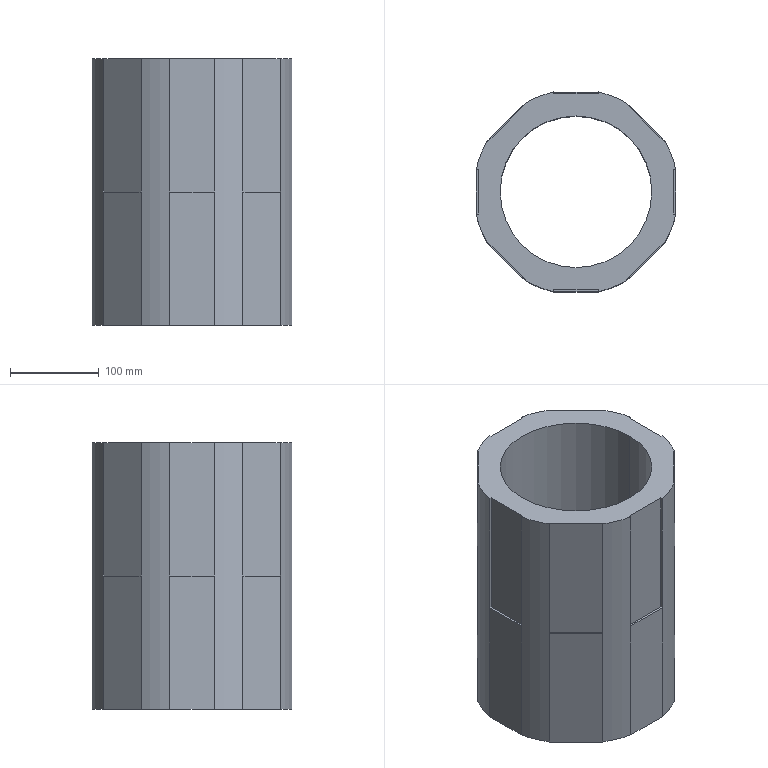Part | SolidWorks | features BaseBody 1 | 1 solid | 52 faces | box 224.499 x 224.499 x 300 mm | volume 5216561 mm3 | plane 42 | cylinder 10 | commonest cylinder face diameters 230 x8 170.4 x2
STEP:
#1=CARTESIAN_POINT('',(2951.757,1619.154,150.));
#2=VERTEX_POINT('',#1);
#3=CARTESIAN_POINT('',(3122.157,1619.154,150.));
#4=VERTEX_POINT('',#3);
#5=CARTESIAN_POINT('',(3036.957,1619.154,150.));
#6=DIRECTION('',(0.,0.,1.));
#7=DIRECTION('',(1.,0.,0.));
#8=AXIS2_PLACEMENT_3D('',#5,#6,#7);
#9=CIRCLE('',#8,85.2);
#10=EDGE_CURVE('',#2,#4,#9,.T.);
#11=ORIENTED_EDGE('',*,*,#10,.T.);
#12=CARTESIAN_POINT('',(3122.157,1619.154,-150.));
#13=VERTEX_POINT('',#12);
#14=CARTESIAN_POINT('',(3122.157,1619.154,150.));
#15=DIRECTION('',(0.,0.,-1.));
#16=VECTOR('',#15,1000.);
#17=LINE('',#14,#16);
#18=EDGE_CURVE('',#4,#13,#17,.T.);
#19=ORIENTED_EDGE('',*,*,#18,.T.);
#20=CARTESIAN_POINT('',(2951.757,1619.154,-150.));
#21=VERTEX_POINT('',#20);
#22=CARTESIAN_POINT('',(3036.957,1619.154,-150.));
#23=DIRECTION('',(0.,0.,1.));
#24=DIRECTION('',(1.,0.,0.));
#25=AXIS2_PLACEMENT_3D('',#22,#23,#24);
#26=CIRCLE('',#25,85.2);
#27=EDGE_CURVE('',#21,#13,#26,.T.);
#28=ORIENTED_EDGE('',*,*,#27,.F.);
#29=CARTESIAN_POINT('',(2951.757,1619.154,150.));
#30=DIRECTION('',(0.,0.,-1.));
#31=VECTOR('',#30,1000.);
#32=LINE('',#29,#31);
#33=EDGE_CURVE('',#2,#21,#32,.T.);
#34=ORIENTED_EDGE('',*,*,#33,.F.);
#35=EDGE_LOOP('',(#11,#19,#28,#34));
#36=FACE_OUTER_BOUND('',#35,.T.);
#37=CARTESIAN_POINT('',(3036.957,1619.154,150.));
#38=DIRECTION('',(0.,0.,-1.));
#39=DIRECTION('',(-1.,0.,0.));
#40=AXIS2_PLACEMENT_3D('',#37,#38,#39);
#41=CYLINDRICAL_SURFACE('',#40,85.2);
#42=ADVANCED_FACE('',(#36),#41,.F.);
#43=CARTESIAN_POINT('',(2979.668,1718.869,0.));
#44=VERTEX_POINT('',#43);
#45=CARTESIAN_POINT('',(2980.388,1718.149,0.));
#46=VERTEX_POINT('',#45);
#47=CARTESIAN_POINT('',(2979.668,1718.869,0.));
#48=DIRECTION('',(0.7071,-0.7071,0.));
#49=VECTOR('',#48,1000.);
#50=LINE('',#47,#49);
#51=EDGE_CURVE('',#44,#46,#50,.T.);
#52=ORIENTED_EDGE('',*,*,#51,.T.);
#53=CARTESIAN_POINT('',(2980.388,1718.149,150.));
#54=VERTEX_POINT('',#53);
#55=CARTESIAN_POINT('',(2980.388,1718.149,150.));
#56=DIRECTION('',(0.,0.,-1.));
#57=VECTOR('',#56,1000.);
#58=LINE('',#55,#57);
#59=EDGE_CURVE('',#54,#46,#58,.T.);
#60=ORIENTED_EDGE('',*,*,#59,.F.);
#61=CARTESIAN_POINT('',(2979.668,1718.869,150.));
#62=VERTEX_POINT('',#61);
#63=CARTESIAN_POINT('',(2979.668,1718.869,150.));
#64=DIRECTION('',(0.7071,-0.7071,0.));
#65=VECTOR('',#64,1000.);
#66=LINE('',#63,#65);
#67=EDGE_CURVE('',#62,#54,#66,.T.);
#68=ORIENTED_EDGE('',*,*,#67,.F.);
#69=CARTESIAN_POINT('',(2979.668,1718.869,150.));
#70=DIRECTION('',(0.,0.,-1.));
#71=VECTOR('',#70,1000.);
#72=LINE('',#69,#71);
#73=EDGE_CURVE('',#62,#44,#72,.T.);
#74=ORIENTED_EDGE('',*,*,#73,.T.);
#75=EDGE_LOOP('',(#52,#60,#68,#74));
#76=FACE_OUTER_BOUND('',#75,.T.);
#77=CARTESIAN_POINT('',(2979.668,1718.869,150.));
#78=DIRECTION('',(0.7071,0.7071,0.));
#79=DIRECTION('',(-0.7071,0.7071,0.));
#80=AXIS2_PLACEMENT_3D('',#77,#78,#79);
#81=PLANE('',#80);
#82=ADVANCED_FACE('',(#76),#81,.F.);
#83=CARTESIAN_POINT('',(2937.962,1675.723,0.));
#84=VERTEX_POINT('',#83);
#85=CARTESIAN_POINT('',(2980.388,1718.149,0.));
#86=DIRECTION('',(-0.7071,-0.7071,0.));
#87=VECTOR('',#86,1000.);
#88=LINE('',#85,#87);
#89=EDGE_CURVE('',#46,#84,#88,.T.);
#90=ORIENTED_EDGE('',*,*,#89,.T.);
#91=CARTESIAN_POINT('',(2937.962,1675.723,150.));
#92=VERTEX_POINT('',#91);
#93=CARTESIAN_POINT('',(2937.962,1675.723,150.));
#94=DIRECTION('',(0.,0.,-1.));
#95=VECTOR('',#94,1000.);
#96=LINE('',#93,#95);
#97=EDGE_CURVE('',#92,#84,#96,.T.);
#98=ORIENTED_EDGE('',*,*,#97,.F.);
#99=CARTESIAN_POINT('',(2980.388,1718.149,150.));
#100=DIRECTION('',(-0.7071,-0.7071,0.));
#101=VECTOR('',#100,1000.);
#102=LINE('',#99,#101);
#103=EDGE_CURVE('',#54,#92,#102,.T.);
#104=ORIENTED_EDGE('',*,*,#103,.F.);
#105=ORIENTED_EDGE('',*,*,#59,.T.);
#106=EDGE_LOOP('',(#90,#98,#104,#105));
#107=FACE_OUTER_BOUND('',#106,.T.);
#108=CARTESIAN_POINT('',(2980.388,1718.149,150.));
#109=DIRECTION('',(0.7071,-0.7071,0.));
#110=DIRECTION('',(0.7071,0.7071,0.));
#111=AXIS2_PLACEMENT_3D('',#108,#109,#110);
#112=PLANE('',#111);
#113=ADVANCED_FACE('',(#107),#112,.F.);
#114=CARTESIAN_POINT('',(2937.242,1676.443,0.));
#115=VERTEX_POINT('',#114);
#116=CARTESIAN_POINT('',(2937.962,1675.723,0.));
#117=DIRECTION('',(-0.7071,0.7071,0.));
#118=VECTOR('',#117,1000.);
#119=LINE('',#116,#118);
#120=EDGE_CURVE('',#84,#115,#119,.T.);
#121=ORIENTED_EDGE('',*,*,#120,.T.);
#122=CARTESIAN_POINT('',(2937.242,1676.443,150.));
#123=VERTEX_POINT('',#122);
#124=CARTESIAN_POINT('',(2937.242,1676.443,150.));
#125=DIRECTION('',(0.,0.,-1.));
#126=VECTOR('',#125,1000.);
#127=LINE('',#124,#126);
#128=EDGE_CURVE('',#123,#115,#127,.T.);
#129=ORIENTED_EDGE('',*,*,#128,.F.);
#130=CARTESIAN_POINT('',(2937.962,1675.723,150.));
#131=DIRECTION('',(-0.7071,0.7071,0.));
#132=VECTOR('',#131,1000.);
#133=LINE('',#130,#132);
#134=EDGE_CURVE('',#92,#123,#133,.T.);
#135=ORIENTED_EDGE('',*,*,#134,.F.);
#136=ORIENTED_EDGE('',*,*,#97,.T.);
#137=EDGE_LOOP('',(#121,#129,#135,#136));
#138=FACE_OUTER_BOUND('',#137,.T.);
#139=CARTESIAN_POINT('',(2937.962,1675.723,150.));
#140=DIRECTION('',(-0.7071,-0.7071,0.));
#141=DIRECTION('',(0.7071,-0.7071,0.));
#142=AXIS2_PLACEMENT_3D('',#139,#140,#141);
#143=PLANE('',#142);
#144=ADVANCED_FACE('',(#138),#143,.F.);
#145=CARTESIAN_POINT('',(2924.707,1644.154,0.));
#146=VERTEX_POINT('',#145);
#147=CARTESIAN_POINT('',(2926.957,1644.154,0.));
#148=VERTEX_POINT('',#147);
#149=CARTESIAN_POINT('',(2924.707,1644.154,0.));
#150=DIRECTION('',(1.,0.,0.));
#151=VECTOR('',#150,1000.);
#152=LINE('',#149,#151);
#153=EDGE_CURVE('',#146,#148,#152,.T.);
#154=ORIENTED_EDGE('',*,*,#153,.T.);
#155=CARTESIAN_POINT('',(2926.957,1644.154,150.));
#156=VERTEX_POINT('',#155);
#157=CARTESIAN_POINT('',(2926.957,1644.154,150.));
#158=DIRECTION('',(0.,0.,-1.));
#159=VECTOR('',#158,1000.);
#160=LINE('',#157,#159);
#161=EDGE_CURVE('',#156,#148,#160,.T.);
#162=ORIENTED_EDGE('',*,*,#161,.F.);
#163=CARTESIAN_POINT('',(2924.707,1644.154,150.));
#164=VERTEX_POINT('',#163);
#165=CARTESIAN_POINT('',(2924.707,1644.154,150.));
#166=DIRECTION('',(1.,0.,0.));
#167=VECTOR('',#166,1000.);
#168=LINE('',#165,#167);
#169=EDGE_CURVE('',#164,#156,#168,.T.);
#170=ORIENTED_EDGE('',*,*,#169,.F.);
#171=CARTESIAN_POINT('',(2924.707,1644.154,150.));
#172=DIRECTION('',(0.,0.,-1.));
#173=VECTOR('',#172,1000.);
#174=LINE('',#171,#173);
#175=EDGE_CURVE('',#164,#146,#174,.T.);
#176=ORIENTED_EDGE('',*,*,#175,.T.);
#177=EDGE_LOOP('',(#154,#162,#170,#176));
#178=FACE_OUTER_BOUND('',#177,.T.);
#179=CARTESIAN_POINT('',(2924.707,1644.154,150.));
#180=DIRECTION('',(0.,1.,0.));
#181=DIRECTION('',(0.,0.,1.));
#182=AXIS2_PLACEMENT_3D('',#179,#180,#181);
#183=PLANE('',#182);
#184=ADVANCED_FACE('',(#178),#183,.F.);
#185=CARTESIAN_POINT('',(2926.957,1594.154,0.));
#186=VERTEX_POINT('',#185);
#187=CARTESIAN_POINT('',(2926.957,1644.154,0.));
#188=DIRECTION('',(0.,-1.,0.));
#189=VECTOR('',#188,1000.);
#190=LINE('',#187,#189);
#191=EDGE_CURVE('',#148,#186,#190,.T.);
#192=ORIENTED_EDGE('',*,*,#191,.T.);
#193=CARTESIAN_POINT('',(2926.957,1594.154,150.));
#194=VERTEX_POINT('',#193);
#195=CARTESIAN_POINT('',(2926.957,1594.154,150.));
#196=DIRECTION('',(0.,0.,-1.));
#197=VECTOR('',#196,1000.);
#198=LINE('',#195,#197);
#199=EDGE_CURVE('',#194,#186,#198,.T.);
#200=ORIENTED_EDGE('',*,*,#199,.F.);
#201=CARTESIAN_POINT('',(2926.957,1644.154,150.));
#202=DIRECTION('',(0.,-1.,0.));
#203=VECTOR('',#202,1000.);
#204=LINE('',#201,#203);
#205=EDGE_CURVE('',#156,#194,#204,.T.);
#206=ORIENTED_EDGE('',*,*,#205,.F.);
#207=ORIENTED_EDGE('',*,*,#161,.T.);
#208=EDGE_LOOP('',(#192,#200,#206,#207));
#209=FACE_OUTER_BOUND('',#208,.T.);
#210=CARTESIAN_POINT('',(2926.957,1644.154,150.));
#211=DIRECTION('',(1.,0.,0.));
#212=DIRECTION('',(0.,0.,-1.));
#213=AXIS2_PLACEMENT_3D('',#210,#211,#212);
#214=PLANE('',#213);
#215=ADVANCED_FACE('',(#209),#214,.F.);
#216=CARTESIAN_POINT('',(2924.707,1594.154,0.));
#217=VERTEX_POINT('',#216);
#218=CARTESIAN_POINT('',(2926.957,1594.154,0.));
#219=DIRECTION('',(-1.,0.,0.));
#220=VECTOR('',#219,1000.);
#221=LINE('',#218,#220);
#222=EDGE_CURVE('',#186,#217,#221,.T.);
#223=ORIENTED_EDGE('',*,*,#222,.T.);
#224=CARTESIAN_POINT('',(2924.707,1594.154,150.));
#225=VERTEX_POINT('',#224);
#226=CARTESIAN_POINT('',(2924.707,1594.154,150.));
#227=DIRECTION('',(0.,0.,-1.));
#228=VECTOR('',#227,1000.);
#229=LINE('',#226,#228);
#230=EDGE_CURVE('',#225,#217,#229,.T.);
#231=ORIENTED_EDGE('',*,*,#230,.F.);
#232=CARTESIAN_POINT('',(2926.957,1594.154,150.));
#233=DIRECTION('',(-1.,0.,0.));
#234=VECTOR('',#233,1000.);
#235=LINE('',#232,#234);
#236=EDGE_CURVE('',#194,#225,#235,.T.);
#237=ORIENTED_EDGE('',*,*,#236,.F.);
#238=ORIENTED_EDGE('',*,*,#199,.T.);
#239=EDGE_LOOP('',(#223,#231,#237,#238));
#240=FACE_OUTER_BOUND('',#239,.T.);
#241=CARTESIAN_POINT('',(2926.957,1594.154,150.));
#242=DIRECTION('',(0.,-1.,0.));
#243=DIRECTION('',(0.,0.,-1.));
#244=AXIS2_PLACEMENT_3D('',#241,#242,#243);
#245=PLANE('',#244);
#246=ADVANCED_FACE('',(#240),#245,.F.);
#247=CARTESIAN_POINT('',(2937.242,1561.866,0.));
#248=VERTEX_POINT('',#247);
#249=CARTESIAN_POINT('',(2937.962,1562.586,0.));
#250=VERTEX_POINT('',#249);
#251=CARTESIAN_POINT('',(2937.242,1561.866,0.));
#252=DIRECTION('',(0.7071,0.7071,0.));
#253=VECTOR('',#252,1000.);
#254=LINE('',#251,#253);
#255=EDGE_CURVE('',#248,#250,#254,.T.);
#256=ORIENTED_EDGE('',*,*,#255,.T.);
#257=CARTESIAN_POINT('',(2937.962,1562.586,150.));
#258=VERTEX_POINT('',#257);
#259=CARTESIAN_POINT('',(2937.962,1562.586,150.));
#260=DIRECTION('',(0.,0.,-1.));
#261=VECTOR('',#260,1000.);
#262=LINE('',#259,#261);
#263=EDGE_CURVE('',#258,#250,#262,.T.);
#264=ORIENTED_EDGE('',*,*,#263,.F.);
#265=CARTESIAN_POINT('',(2937.242,1561.866,150.));
#266=VERTEX_POINT('',#265);
#267=CARTESIAN_POINT('',(2937.242,1561.866,150.));
#268=DIRECTION('',(0.7071,0.7071,0.));
#269=VECTOR('',#268,1000.);
#270=LINE('',#267,#269);
#271=EDGE_CURVE('',#266,#258,#270,.T.);
#272=ORIENTED_EDGE('',*,*,#271,.F.);
#273=CARTESIAN_POINT('',(2937.242,1561.866,150.));
#274=DIRECTION('',(0.,0.,-1.));
#275=VECTOR('',#274,1000.);
#276=LINE('',#273,#275);
#277=EDGE_CURVE('',#266,#248,#276,.T.);
#278=ORIENTED_EDGE('',*,*,#277,.T.);
#279=EDGE_LOOP('',(#256,#264,#272,#278));
#280=FACE_OUTER_BOUND('',#279,.T.);
#281=CARTESIAN_POINT('',(2937.242,1561.866,150.));
#282=DIRECTION('',(-0.7071,0.7071,0.));
#283=DIRECTION('',(-0.7071,-0.7071,0.));
#284=AXIS2_PLACEMENT_3D('',#281,#282,#283);
#285=PLANE('',#284);
#286=ADVANCED_FACE('',(#280),#285,.F.);
#287=CARTESIAN_POINT('',(2980.388,1520.159,0.));
#288=VERTEX_POINT('',#287);
#289=CARTESIAN_POINT('',(2937.962,1562.586,0.));
#290=DIRECTION('',(0.7071,-0.7071,0.));
#291=VECTOR('',#290,1000.);
#292=LINE('',#289,#291);
#293=EDGE_CURVE('',#250,#288,#292,.T.);
#294=ORIENTED_EDGE('',*,*,#293,.T.);
#295=CARTESIAN_POINT('',(2980.388,1520.159,150.));
#296=VERTEX_POINT('',#295);
#297=CARTESIAN_POINT('',(2980.388,1520.159,150.));
#298=DIRECTION('',(0.,0.,-1.));
#299=VECTOR('',#298,1000.);
#300=LINE('',#297,#299);
#301=EDGE_CURVE('',#296,#288,#300,.T.);
#302=ORIENTED_EDGE('',*,*,#301,.F.);
#303=CARTESIAN_POINT('',(2937.962,1562.586,150.));
#304=DIRECTION('',(0.7071,-0.7071,0.));
#305=VECTOR('',#304,1000.);
#306=LINE('',#303,#305);
#307=EDGE_CURVE('',#258,#296,#306,.T.);
#308=ORIENTED_EDGE('',*,*,#307,.F.);
#309=ORIENTED_EDGE('',*,*,#263,.T.);
#310=EDGE_LOOP('',(#294,#302,#308,#309));
#311=FACE_OUTER_BOUND('',#310,.T.);
#312=CARTESIAN_POINT('',(2937.962,1562.586,150.));
#313=DIRECTION('',(0.7071,0.7071,0.));
#314=DIRECTION('',(-0.7071,0.7071,0.));
#315=AXIS2_PLACEMENT_3D('',#312,#313,#314);
#316=PLANE('',#315);
#317=ADVANCED_FACE('',(#311),#316,.F.);
#318=CARTESIAN_POINT('',(2979.668,1519.439,0.));
#319=VERTEX_POINT('',#318);
#320=CARTESIAN_POINT('',(2980.388,1520.159,0.));
#321=DIRECTION('',(-0.7071,-0.7071,0.));
#322=VECTOR('',#321,1000.);
#323=LINE('',#320,#322);
#324=EDGE_CURVE('',#288,#319,#323,.T.);
#325=ORIENTED_EDGE('',*,*,#324,.T.);
#326=CARTESIAN_POINT('',(2979.668,1519.439,150.));
#327=VERTEX_POINT('',#326);
#328=CARTESIAN_POINT('',(2979.668,1519.439,150.));
#329=DIRECTION('',(0.,0.,-1.));
#330=VECTOR('',#329,1000.);
#331=LINE('',#328,#330);
#332=EDGE_CURVE('',#327,#319,#331,.T.);
#333=ORIENTED_EDGE('',*,*,#332,.F.);
#334=CARTESIAN_POINT('',(2980.388,1520.159,150.));
#335=DIRECTION('',(-0.7071,-0.7071,0.));
#336=VECTOR('',#335,1000.);
#337=LINE('',#334,#336);
#338=EDGE_CURVE('',#296,#327,#337,.T.);
#339=ORIENTED_EDGE('',*,*,#338,.F.);
#340=ORIENTED_EDGE('',*,*,#301,.T.);
#341=EDGE_LOOP('',(#325,#333,#339,#340));
#342=FACE_OUTER_BOUND('',#341,.T.);
#343=CARTESIAN_POINT('',(2980.388,1520.159,150.));
#344=DIRECTION('',(0.7071,-0.7071,0.));
#345=DIRECTION('',(0.7071,0.7071,0.));
#346=AXIS2_PLACEMENT_3D('',#343,#344,#345);
#347=PLANE('',#346);
#348=ADVANCED_FACE('',(#342),#347,.F.);
#349=CARTESIAN_POINT('',(3094.245,1718.869,150.));
#350=VERTEX_POINT('',#349);
#351=CARTESIAN_POINT('',(3061.957,1731.404,150.));
#352=VERTEX_POINT('',#351);
#353=CARTESIAN_POINT('',(3036.957,1619.154,150.));
#354=DIRECTION('',(0.,0.,1.));
#355=DIRECTION('',(1.,0.,0.));
#356=AXIS2_PLACEMENT_3D('',#353,#354,#355);
#357=CIRCLE('',#356,115.);
#358=EDGE_CURVE('',#350,#352,#357,.T.);
#359=ORIENTED_EDGE('',*,*,#358,.T.);
#360=CARTESIAN_POINT('',(3061.957,1729.154,150.));
#361=VERTEX_POINT('',#360);
#362=CARTESIAN_POINT('',(3061.957,1731.404,150.));
#363=DIRECTION('',(0.,-1.,0.));
#364=VECTOR('',#363,1000.);
#365=LINE('',#362,#364);
#366=EDGE_CURVE('',#352,#361,#365,.T.);
#367=ORIENTED_EDGE('',*,*,#366,.T.);
#368=CARTESIAN_POINT('',(3011.957,1729.154,150.));
#369=VERTEX_POINT('',#368);
#370=CARTESIAN_POINT('',(3061.957,1729.154,150.));
#371=DIRECTION('',(-1.,0.,0.));
#372=VECTOR('',#371,1000.);
#373=LINE('',#370,#372);
#374=EDGE_CURVE('',#361,#369,#373,.T.);
#375=ORIENTED_EDGE('',*,*,#374,.T.);
#376=CARTESIAN_POINT('',(3011.957,1731.404,150.));
#377=VERTEX_POINT('',#376);
#378=CARTESIAN_POINT('',(3011.957,1729.154,150.));
#379=DIRECTION('',(0.,1.,0.));
#380=VECTOR('',#379,1000.);
#381=LINE('',#378,#380);
#382=EDGE_CURVE('',#369,#377,#381,.T.);
#383=ORIENTED_EDGE('',*,*,#382,.T.);
#384=CARTESIAN_POINT('',(3036.957,1619.154,150.));
#385=DIRECTION('',(0.,0.,1.));
#386=DIRECTION('',(1.,0.,0.));
#387=AXIS2_PLACEMENT_3D('',#384,#385,#386);
#388=CIRCLE('',#387,115.);
#389=EDGE_CURVE('',#377,#62,#388,.T.);
#390=ORIENTED_EDGE('',*,*,#389,.T.);
#391=ORIENTED_EDGE('',*,*,#67,.T.);
#392=ORIENTED_EDGE('',*,*,#103,.T.);
#393=ORIENTED_EDGE('',*,*,#134,.T.);
#394=CARTESIAN_POINT('',(3036.957,1619.154,150.));
#395=DIRECTION('',(0.,0.,1.));
#396=DIRECTION('',(1.,0.,0.));
#397=AXIS2_PLACEMENT_3D('',#394,#395,#396);
#398=CIRCLE('',#397,115.);
#399=EDGE_CURVE('',#123,#164,#398,.T.);
#400=ORIENTED_EDGE('',*,*,#399,.T.);
#401=ORIENTED_EDGE('',*,*,#169,.T.);
#402=ORIENTED_EDGE('',*,*,#205,.T.);
#403=ORIENTED_EDGE('',*,*,#236,.T.);
#404=CARTESIAN_POINT('',(3036.957,1619.154,150.));
#405=DIRECTION('',(0.,0.,1.));
#406=DIRECTION('',(1.,0.,0.));
#407=AXIS2_PLACEMENT_3D('',#404,#405,#406);
#408=CIRCLE('',#407,115.);
#409=EDGE_CURVE('',#225,#266,#408,.T.);
#410=ORIENTED_EDGE('',*,*,#409,.T.);
#411=ORIENTED_EDGE('',*,*,#271,.T.);
#412=ORIENTED_EDGE('',*,*,#307,.T.);
#413=ORIENTED_EDGE('',*,*,#338,.T.);
#414=CARTESIAN_POINT('',(3011.957,1506.905,150.));
#415=VERTEX_POINT('',#414);
#416=CARTESIAN_POINT('',(3036.957,1619.154,150.));
#417=DIRECTION('',(0.,0.,1.));
#418=DIRECTION('',(1.,0.,0.));
#419=AXIS2_PLACEMENT_3D('',#416,#417,#418);
#420=CIRCLE('',#419,115.);
#421=EDGE_CURVE('',#327,#415,#420,.T.);
#422=ORIENTED_EDGE('',*,*,#421,.T.);
#423=CARTESIAN_POINT('',(3011.957,1509.154,150.));
#424=VERTEX_POINT('',#423);
#425=CARTESIAN_POINT('',(3011.957,1506.905,150.));
#426=DIRECTION('',(0.,1.,0.));
#427=VECTOR('',#426,1000.);
#428=LINE('',#425,#427);
#429=EDGE_CURVE('',#415,#424,#428,.T.);
#430=ORIENTED_EDGE('',*,*,#429,.T.);
#431=CARTESIAN_POINT('',(3061.957,1509.154,150.));
#432=VERTEX_POINT('',#431);
#433=CARTESIAN_POINT('',(3011.957,1509.154,150.));
#434=DIRECTION('',(1.,0.,0.));
#435=VECTOR('',#434,1000.);
#436=LINE('',#433,#435);
#437=EDGE_CURVE('',#424,#432,#436,.T.);
#438=ORIENTED_EDGE('',*,*,#437,.T.);
#439=CARTESIAN_POINT('',(3061.957,1506.905,150.));
#440=VERTEX_POINT('',#439);
#441=CARTESIAN_POINT('',(3061.957,1509.154,150.));
#442=DIRECTION('',(0.,-1.,0.));
#443=VECTOR('',#442,1000.);
#444=LINE('',#441,#443);
#445=EDGE_CURVE('',#432,#440,#444,.T.);
#446=ORIENTED_EDGE('',*,*,#445,.T.);
#447=CARTESIAN_POINT('',(3094.245,1519.439,150.));
#448=VERTEX_POINT('',#447);
#449=CARTESIAN_POINT('',(3036.957,1619.154,150.));
#450=DIRECTION('',(0.,0.,1.));
#451=DIRECTION('',(1.,0.,0.));
#452=AXIS2_PLACEMENT_3D('',#449,#450,#451);
#453=CIRCLE('',#452,115.);
#454=EDGE_CURVE('',#440,#448,#453,.T.);
#455=ORIENTED_EDGE('',*,*,#454,.T.);
#456=CARTESIAN_POINT('',(3093.525,1520.159,150.));
#457=VERTEX_POINT('',#456);
#458=CARTESIAN_POINT('',(3094.245,1519.439,150.));
#459=DIRECTION('',(-0.7071,0.7071,0.));
#460=VECTOR('',#459,1000.);
#461=LINE('',#458,#460);
#462=EDGE_CURVE('',#448,#457,#461,.T.);
#463=ORIENTED_EDGE('',*,*,#462,.T.);
#464=CARTESIAN_POINT('',(3135.952,1562.586,150.));
#465=VERTEX_POINT('',#464);
#466=CARTESIAN_POINT('',(3093.525,1520.159,150.));
#467=DIRECTION('',(0.7071,0.7071,0.));
#468=VECTOR('',#467,1000.);
#469=LINE('',#466,#468);
#470=EDGE_CURVE('',#457,#465,#469,.T.);
#471=ORIENTED_EDGE('',*,*,#470,.T.);
#472=CARTESIAN_POINT('',(3136.672,1561.866,150.));
#473=VERTEX_POINT('',#472);
#474=CARTESIAN_POINT('',(3135.952,1562.586,150.));
#475=DIRECTION('',(0.7071,-0.7071,0.));
#476=VECTOR('',#475,1000.);
#477=LINE('',#474,#476);
#478=EDGE_CURVE('',#465,#473,#477,.T.);
#479=ORIENTED_EDGE('',*,*,#478,.T.);
#480=CARTESIAN_POINT('',(3149.207,1594.154,150.));
#481=VERTEX_POINT('',#480);
#482=CARTESIAN_POINT('',(3036.957,1619.154,150.));
#483=DIRECTION('',(0.,0.,1.));
#484=DIRECTION('',(1.,0.,0.));
#485=AXIS2_PLACEMENT_3D('',#482,#483,#484);
#486=CIRCLE('',#485,115.);
#487=EDGE_CURVE('',#473,#481,#486,.T.);
#488=ORIENTED_EDGE('',*,*,#487,.T.);
#489=CARTESIAN_POINT('',(3146.957,1594.154,150.));
#490=VERTEX_POINT('',#489);
#491=CARTESIAN_POINT('',(3149.207,1594.154,150.));
#492=DIRECTION('',(-1.,0.,0.));
#493=VECTOR('',#492,1000.);
#494=LINE('',#491,#493);
#495=EDGE_CURVE('',#481,#490,#494,.T.);
#496=ORIENTED_EDGE('',*,*,#495,.T.);
#497=CARTESIAN_POINT('',(3146.957,1644.154,150.));
#498=VERTEX_POINT('',#497);
#499=CARTESIAN_POINT('',(3146.957,1594.154,150.));
#500=DIRECTION('',(0.,1.,0.));
#501=VECTOR('',#500,1000.);
#502=LINE('',#499,#501);
#503=EDGE_CURVE('',#490,#498,#502,.T.);
#504=ORIENTED_EDGE('',*,*,#503,.T.);
#505=CARTESIAN_POINT('',(3149.207,1644.154,150.));
#506=VERTEX_POINT('',#505);
#507=CARTESIAN_POINT('',(3146.957,1644.154,150.));
#508=DIRECTION('',(1.,0.,0.));
#509=VECTOR('',#508,1000.);
#510=LINE('',#507,#509);
#511=EDGE_CURVE('',#498,#506,#510,.T.);
#512=ORIENTED_EDGE('',*,*,#511,.T.);
#513=CARTESIAN_POINT('',(3136.672,1676.443,150.));
#514=VERTEX_POINT('',#513);
#515=CARTESIAN_POINT('',(3036.957,1619.154,150.));
#516=DIRECTION('',(0.,0.,1.));
#517=DIRECTION('',(1.,0.,0.));
#518=AXIS2_PLACEMENT_3D('',#515,#516,#517);
#519=CIRCLE('',#518,115.);
#520=EDGE_CURVE('',#506,#514,#519,.T.);
#521=ORIENTED_EDGE('',*,*,#520,.T.);
#522=CARTESIAN_POINT('',(3135.952,1675.723,150.));
#523=VERTEX_POINT('',#522);
#524=CARTESIAN_POINT('',(3136.672,1676.443,150.));
#525=DIRECTION('',(-0.7071,-0.7071,0.));
#526=VECTOR('',#525,1000.);
#527=LINE('',#524,#526);
#528=EDGE_CURVE('',#514,#523,#527,.T.);
#529=ORIENTED_EDGE('',*,*,#528,.T.);
#530=CARTESIAN_POINT('',(3093.525,1718.149,150.));
#531=VERTEX_POINT('',#530);
#532=CARTESIAN_POINT('',(3135.952,1675.723,150.));
#533=DIRECTION('',(-0.7071,0.7071,0.));
#534=VECTOR('',#533,1000.);
#535=LINE('',#532,#534);
#536=EDGE_CURVE('',#523,#531,#535,.T.);
#537=ORIENTED_EDGE('',*,*,#536,.T.);
#538=CARTESIAN_POINT('',(3093.525,1718.149,150.));
#539=DIRECTION('',(0.7071,0.7071,0.));
#540=VECTOR('',#539,1000.);
#541=LINE('',#538,#540);
#542=EDGE_CURVE('',#531,#350,#541,.T.);
#543=ORIENTED_EDGE('',*,*,#542,.T.);
#544=EDGE_LOOP('',(#359,#367,#375,#383,#390,#391,#392,#393,#400,#401,#402,#403,#410,#411,#412,#413,#422,#430,#438,#446,#455,#463,#471,#479,#488,#496,#504,#512,#521,#529,#537,#543));
#545=FACE_OUTER_BOUND('',#544,.T.);
#546=ORIENTED_EDGE('',*,*,#10,.F.);
#547=CARTESIAN_POINT('',(3036.957,1619.154,150.));
#548=DIRECTION('',(0.,0.,1.));
#549=DIRECTION('',(1.,0.,0.));
#550=AXIS2_PLACEMENT_3D('',#547,#548,#549);
#551=CIRCLE('',#550,85.2);
#552=EDGE_CURVE('',#4,#2,#551,.T.);
#553=ORIENTED_EDGE('',*,*,#552,.F.);
#554=EDGE_LOOP('',(#546,#553));
#555=FACE_BOUND('',#554,.T.);
#556=CARTESIAN_POINT('',(3036.957,1619.154,150.));
#557=DIRECTION('',(0.,0.,1.));
#558=DIRECTION('',(1.,0.,0.));
#559=AXIS2_PLACEMENT_3D('',#556,#557,#558);
#560=PLANE('',#559);
#561=ADVANCED_FACE('',(#545,#555),#560,.T.);
#562=CARTESIAN_POINT('',(3094.245,1718.869,-150.));
#563=VERTEX_POINT('',#562);
#564=CARTESIAN_POINT('',(3061.957,1731.404,-150.));
#565=VERTEX_POINT('',#564);
#566=CARTESIAN_POINT('',(3036.957,1619.154,-150.));
#567=DIRECTION('',(0.,0.,1.));
#568=DIRECTION('',(1.,0.,0.));
#569=AXIS2_PLACEMENT_3D('',#566,#567,#568);
#570=CIRCLE('',#569,115.);
#571=EDGE_CURVE('',#563,#565,#570,.T.);
#572=ORIENTED_EDGE('',*,*,#571,.F.);
#573=CARTESIAN_POINT('',(3136.672,1676.443,-150.));
#574=VERTEX_POINT('',#573);
#575=CARTESIAN_POINT('',(3136.672,1676.443,-150.));
#576=DIRECTION('',(0.7071,-0.7071,0.));
#577=VECTOR('',#576,1000.);
#578=LINE('',#575,#577);
#579=EDGE_CURVE('',#563,#574,#578,.T.);
#580=ORIENTED_EDGE('',*,*,#579,.T.);
#581=CARTESIAN_POINT('',(3149.207,1644.154,-150.));
#582=VERTEX_POINT('',#581);
#583=CARTESIAN_POINT('',(3036.957,1619.154,-150.));
#584=DIRECTION('',(0.,0.,1.));
#585=DIRECTION('',(1.,0.,0.));
#586=AXIS2_PLACEMENT_3D('',#583,#584,#585);
#587=CIRCLE('',#586,115.);
#588=EDGE_CURVE('',#582,#574,#587,.T.);
#589=ORIENTED_EDGE('',*,*,#588,.F.);
#590=CARTESIAN_POINT('',(3149.207,1594.154,-150.));
#591=VERTEX_POINT('',#590);
#592=CARTESIAN_POINT('',(3149.207,1594.154,-150.));
#593=DIRECTION('',(0.,-1.,0.));
#594=VECTOR('',#593,1000.);
#595=LINE('',#592,#594);
#596=EDGE_CURVE('',#582,#591,#595,.T.);
#597=ORIENTED_EDGE('',*,*,#596,.T.);
#598=CARTESIAN_POINT('',(3136.672,1561.866,-150.));
#599=VERTEX_POINT('',#598);
#600=CARTESIAN_POINT('',(3036.957,1619.154,-150.));
#601=DIRECTION('',(0.,0.,1.));
#602=DIRECTION('',(1.,0.,0.));
#603=AXIS2_PLACEMENT_3D('',#600,#601,#602);
#604=CIRCLE('',#603,115.);
#605=EDGE_CURVE('',#599,#591,#604,.T.);
#606=ORIENTED_EDGE('',*,*,#605,.F.);
#607=CARTESIAN_POINT('',(3094.245,1519.439,-150.));
#608=VERTEX_POINT('',#607);
#609=CARTESIAN_POINT('',(3094.245,1519.439,-150.));
#610=DIRECTION('',(-0.7071,-0.7071,0.));
#611=VECTOR('',#610,1000.);
#612=LINE('',#609,#611);
#613=EDGE_CURVE('',#599,#608,#612,.T.);
#614=ORIENTED_EDGE('',*,*,#613,.T.);
#615=CARTESIAN_POINT('',(3061.957,1506.905,-150.));
#616=VERTEX_POINT('',#615);
#617=CARTESIAN_POINT('',(3036.957,1619.154,-150.));
#618=DIRECTION('',(0.,0.,1.));
#619=DIRECTION('',(1.,0.,0.));
#620=AXIS2_PLACEMENT_3D('',#617,#618,#619);
#621=CIRCLE('',#620,115.);
#622=EDGE_CURVE('',#616,#608,#621,.T.);
#623=ORIENTED_EDGE('',*,*,#622,.F.);
#624=CARTESIAN_POINT('',(3011.957,1506.905,-150.));
#625=VERTEX_POINT('',#624);
#626=CARTESIAN_POINT('',(3011.957,1506.905,-150.));
#627=DIRECTION('',(-1.,0.,0.));
#628=VECTOR('',#627,1000.);
#629=LINE('',#626,#628);
#630=EDGE_CURVE('',#616,#625,#629,.T.);
#631=ORIENTED_EDGE('',*,*,#630,.T.);
#632=CARTESIAN_POINT('',(2979.668,1519.439,-150.));
#633=VERTEX_POINT('',#632);
#634=CARTESIAN_POINT('',(3036.957,1619.154,-150.));
#635=DIRECTION('',(0.,0.,1.));
#636=DIRECTION('',(1.,0.,0.));
#637=AXIS2_PLACEMENT_3D('',#634,#635,#636);
#638=CIRCLE('',#637,115.);
#639=EDGE_CURVE('',#633,#625,#638,.T.);
#640=ORIENTED_EDGE('',*,*,#639,.F.);
#641=CARTESIAN_POINT('',(2937.242,1561.866,-150.));
#642=VERTEX_POINT('',#641);
#643=CARTESIAN_POINT('',(2979.668,1519.439,-150.));
#644=DIRECTION('',(-0.7071,0.7071,0.));
#645=VECTOR('',#644,1000.);
#646=LINE('',#643,#645);
#647=EDGE_CURVE('',#633,#642,#646,.T.);
#648=ORIENTED_EDGE('',*,*,#647,.T.);
#649=CARTESIAN_POINT('',(2924.707,1594.154,-150.));
#650=VERTEX_POINT('',#649);
#651=CARTESIAN_POINT('',(3036.957,1619.154,-150.));
#652=DIRECTION('',(0.,0.,1.));
#653=DIRECTION('',(1.,0.,0.));
#654=AXIS2_PLACEMENT_3D('',#651,#652,#653);
#655=CIRCLE('',#654,115.);
#656=EDGE_CURVE('',#650,#642,#655,.T.);
#657=ORIENTED_EDGE('',*,*,#656,.F.);
#658=CARTESIAN_POINT('',(2924.707,1644.154,-150.));
#659=VERTEX_POINT('',#658);
#660=CARTESIAN_POINT('',(2924.707,1594.154,-150.));
#661=DIRECTION('',(0.,1.,0.));
#662=VECTOR('',#661,1000.);
#663=LINE('',#660,#662);
#664=EDGE_CURVE('',#650,#659,#663,.T.);
#665=ORIENTED_EDGE('',*,*,#664,.T.);
#666=CARTESIAN_POINT('',(2937.242,1676.443,-150.));
#667=VERTEX_POINT('',#666);
#668=CARTESIAN_POINT('',(3036.957,1619.154,-150.));
#669=DIRECTION('',(0.,0.,1.));
#670=DIRECTION('',(1.,0.,0.));
#671=AXIS2_PLACEMENT_3D('',#668,#669,#670);
#672=CIRCLE('',#671,115.);
#673=EDGE_CURVE('',#667,#659,#672,.T.);
#674=ORIENTED_EDGE('',*,*,#673,.F.);
#675=CARTESIAN_POINT('',(2979.668,1718.869,-150.));
#676=VERTEX_POINT('',#675);
#677=CARTESIAN_POINT('',(2937.242,1676.443,-150.));
#678=DIRECTION('',(0.7071,0.7071,0.));
#679=VECTOR('',#678,1000.);
#680=LINE('',#677,#679);
#681=EDGE_CURVE('',#667,#676,#680,.T.);
#682=ORIENTED_EDGE('',*,*,#681,.T.);
#683=CARTESIAN_POINT('',(3011.957,1731.404,-150.));
#684=VERTEX_POINT('',#683);
#685=CARTESIAN_POINT('',(3036.957,1619.154,-150.));
#686=DIRECTION('',(0.,0.,1.));
#687=DIRECTION('',(1.,0.,0.));
#688=AXIS2_PLACEMENT_3D('',#685,#686,#687);
#689=CIRCLE('',#688,115.);
#690=EDGE_CURVE('',#684,#676,#689,.T.);
#691=ORIENTED_EDGE('',*,*,#690,.F.);
#692=CARTESIAN_POINT('',(3061.957,1731.404,-150.));
#693=DIRECTION('',(1.,0.,0.));
#694=VECTOR('',#693,1000.);
#695=LINE('',#692,#694);
#696=EDGE_CURVE('',#684,#565,#695,.T.);
#697=ORIENTED_EDGE('',*,*,#696,.T.);
#698=EDGE_LOOP('',(#572,#580,#589,#597,#606,#614,#623,#631,#640,#648,#657,#665,#674,#682,#691,#697));
#699=FACE_OUTER_BOUND('',#698,.T.);
#700=ORIENTED_EDGE('',*,*,#27,.T.);
#701=CARTESIAN_POINT('',(3036.957,1619.154,-150.));
#702=DIRECTION('',(0.,0.,1.));
#703=DIRECTION('',(1.,0.,0.));
#704=AXIS2_PLACEMENT_3D('',#701,#702,#703);
#705=CIRCLE('',#704,85.2);
#706=EDGE_CURVE('',#13,#21,#705,.T.);
#707=ORIENTED_EDGE('',*,*,#706,.T.);
#708=EDGE_LOOP('',(#700,#707));
#709=FACE_BOUND('',#708,.T.);
#710=CARTESIAN_POINT('',(3036.957,1619.154,-150.));
#711=DIRECTION('',(0.,0.,1.));
#712=DIRECTION('',(1.,0.,0.));
#713=AXIS2_PLACEMENT_3D('',#710,#711,#712);
#714=PLANE('',#713);
#715=ADVANCED_FACE('',(#699,#709),#714,.F.);
#716=ORIENTED_EDGE('',*,*,#571,.T.);
#717=CARTESIAN_POINT('',(3061.957,1731.404,0.));
#718=VERTEX_POINT('',#717);
#719=CARTESIAN_POINT('',(3061.957,1731.404,0.));
#720=DIRECTION('',(0.,0.,-1.));
#721=VECTOR('',#720,1000.);
#722=LINE('',#719,#721);
#723=EDGE_CURVE('',#718,#565,#722,.T.);
#724=ORIENTED_EDGE('',*,*,#723,.F.);
#725=CARTESIAN_POINT('',(3061.957,1731.404,150.));
#726=DIRECTION('',(0.,0.,-1.));
#727=VECTOR('',#726,1000.);
#728=LINE('',#725,#727);
#729=EDGE_CURVE('',#352,#718,#728,.T.);
#730=ORIENTED_EDGE('',*,*,#729,.F.);
#731=ORIENTED_EDGE('',*,*,#358,.F.);
#732=CARTESIAN_POINT('',(3094.245,1718.869,0.));
#733=VERTEX_POINT('',#732);
#734=CARTESIAN_POINT('',(3094.245,1718.869,150.));
#735=DIRECTION('',(0.,0.,-1.));
#736=VECTOR('',#735,1000.);
#737=LINE('',#734,#736);
#738=EDGE_CURVE('',#350,#733,#737,.T.);
#739=ORIENTED_EDGE('',*,*,#738,.T.);
#740=CARTESIAN_POINT('',(3094.245,1718.869,0.));
#741=DIRECTION('',(0.,0.,-1.));
#742=VECTOR('',#741,1000.);
#743=LINE('',#740,#742);
#744=EDGE_CURVE('',#733,#563,#743,.T.);
#745=ORIENTED_EDGE('',*,*,#744,.T.);
#746=EDGE_LOOP('',(#716,#724,#730,#731,#739,#745));
#747=FACE_OUTER_BOUND('',#746,.T.);
#748=CARTESIAN_POINT('',(3036.957,1619.154,150.));
#749=DIRECTION('',(0.,0.,-1.));
#750=DIRECTION('',(-1.,0.,0.));
#751=AXIS2_PLACEMENT_3D('',#748,#749,#750);
#752=CYLINDRICAL_SURFACE('',#751,115.);
#753=ADVANCED_FACE('',(#747),#752,.T.);
#754=ORIENTED_EDGE('',*,*,#729,.T.);
#755=CARTESIAN_POINT('',(3061.957,1729.154,0.));
#756=VERTEX_POINT('',#755);
#757=CARTESIAN_POINT('',(3061.957,1729.154,0.));
#758=DIRECTION('',(0.,-1.,0.));
#759=VECTOR('',#758,1000.);
#760=LINE('',#757,#759);
#761=EDGE_CURVE('',#718,#756,#760,.T.);
#762=ORIENTED_EDGE('',*,*,#761,.T.);
#763=CARTESIAN_POINT('',(3061.957,1729.154,150.));
#764=DIRECTION('',(0.,0.,-1.));
#765=VECTOR('',#764,1000.);
#766=LINE('',#763,#765);
#767=EDGE_CURVE('',#361,#756,#766,.T.);
#768=ORIENTED_EDGE('',*,*,#767,.F.);
#769=ORIENTED_EDGE('',*,*,#366,.F.);
#770=EDGE_LOOP('',(#754,#762,#768,#769));
#771=FACE_OUTER_BOUND('',#770,.T.);
#772=CARTESIAN_POINT('',(3061.957,1731.404,150.));
#773=DIRECTION('',(1.,0.,0.));
#774=DIRECTION('',(0.,0.,-1.));
#775=AXIS2_PLACEMENT_3D('',#772,#773,#774);
#776=PLANE('',#775);
#777=ADVANCED_FACE('',(#771),#776,.F.);
#778=ORIENTED_EDGE('',*,*,#767,.T.);
#779=CARTESIAN_POINT('',(3011.957,1729.154,0.));
#780=VERTEX_POINT('',#779);
#781=CARTESIAN_POINT('',(3011.957,1729.154,0.));
#782=DIRECTION('',(-1.,0.,0.));
#783=VECTOR('',#782,1000.);
#784=LINE('',#781,#783);
#785=EDGE_CURVE('',#756,#780,#784,.T.);
#786=ORIENTED_EDGE('',*,*,#785,.T.);
#787=CARTESIAN_POINT('',(3011.957,1729.154,150.));
#788=DIRECTION('',(0.,0.,-1.));
#789=VECTOR('',#788,1000.);
#790=LINE('',#787,#789);
#791=EDGE_CURVE('',#369,#780,#790,.T.);
#792=ORIENTED_EDGE('',*,*,#791,.F.);
#793=ORIENTED_EDGE('',*,*,#374,.F.);
#794=EDGE_LOOP('',(#778,#786,#792,#793));
#795=FACE_OUTER_BOUND('',#794,.T.);
#796=CARTESIAN_POINT('',(3061.957,1729.154,150.));
#797=DIRECTION('',(0.,-1.,0.));
#798=DIRECTION('',(0.,0.,-1.));
#799=AXIS2_PLACEMENT_3D('',#796,#797,#798);
#800=PLANE('',#799);
#801=ADVANCED_FACE('',(#795),#800,.F.);
#802=ORIENTED_EDGE('',*,*,#791,.T.);
#803=CARTESIAN_POINT('',(3011.957,1731.404,0.));
#804=VERTEX_POINT('',#803);
#805=CARTESIAN_POINT('',(3011.957,1731.404,0.));
#806=DIRECTION('',(0.,1.,0.));
#807=VECTOR('',#806,1000.);
#808=LINE('',#805,#807);
#809=EDGE_CURVE('',#780,#804,#808,.T.);
#810=ORIENTED_EDGE('',*,*,#809,.T.);
#811=CARTESIAN_POINT('',(3011.957,1731.404,150.));
#812=DIRECTION('',(0.,0.,-1.));
#813=VECTOR('',#812,1000.);
#814=LINE('',#811,#813);
#815=EDGE_CURVE('',#377,#804,#814,.T.);
#816=ORIENTED_EDGE('',*,*,#815,.F.);
#817=ORIENTED_EDGE('',*,*,#382,.F.);
#818=EDGE_LOOP('',(#802,#810,#816,#817));
#819=FACE_OUTER_BOUND('',#818,.T.);
#820=CARTESIAN_POINT('',(3011.957,1729.154,150.));
#821=DIRECTION('',(-1.,0.,0.));
#822=DIRECTION('',(0.,0.,1.));
#823=AXIS2_PLACEMENT_3D('',#820,#821,#822);
#824=PLANE('',#823);
#825=ADVANCED_FACE('',(#819),#824,.F.);
#826=ORIENTED_EDGE('',*,*,#690,.T.);
#827=CARTESIAN_POINT('',(2979.668,1718.869,0.));
#828=DIRECTION('',(0.,0.,-1.));
#829=VECTOR('',#828,1000.);
#830=LINE('',#827,#829);
#831=EDGE_CURVE('',#44,#676,#830,.T.);
#832=ORIENTED_EDGE('',*,*,#831,.F.);
#833=ORIENTED_EDGE('',*,*,#73,.F.);
#834=ORIENTED_EDGE('',*,*,#389,.F.);
#835=ORIENTED_EDGE('',*,*,#815,.T.);
#836=CARTESIAN_POINT('',(3011.957,1731.404,0.));
#837=DIRECTION('',(0.,0.,-1.));
#838=VECTOR('',#837,1000.);
#839=LINE('',#836,#838);
#840=EDGE_CURVE('',#804,#684,#839,.T.);
#841=ORIENTED_EDGE('',*,*,#840,.T.);
#842=EDGE_LOOP('',(#826,#832,#833,#834,#835,#841));
#843=FACE_OUTER_BOUND('',#842,.T.);
#844=CARTESIAN_POINT('',(3036.957,1619.154,150.));
#845=DIRECTION('',(0.,0.,-1.));
#846=DIRECTION('',(-1.,0.,0.));
#847=AXIS2_PLACEMENT_3D('',#844,#845,#846);
#848=CYLINDRICAL_SURFACE('',#847,115.);
#849=ADVANCED_FACE('',(#843),#848,.T.);
#850=ORIENTED_EDGE('',*,*,#673,.T.);
#851=CARTESIAN_POINT('',(2924.707,1644.154,0.));
#852=DIRECTION('',(0.,0.,-1.));
#853=VECTOR('',#852,1000.);
#854=LINE('',#851,#853);
#855=EDGE_CURVE('',#146,#659,#854,.T.);
#856=ORIENTED_EDGE('',*,*,#855,.F.);
#857=ORIENTED_EDGE('',*,*,#175,.F.);
#858=ORIENTED_EDGE('',*,*,#399,.F.);
#859=ORIENTED_EDGE('',*,*,#128,.T.);
#860=CARTESIAN_POINT('',(2937.242,1676.443,0.));
#861=DIRECTION('',(0.,0.,-1.));
#862=VECTOR('',#861,1000.);
#863=LINE('',#860,#862);
#864=EDGE_CURVE('',#115,#667,#863,.T.);
#865=ORIENTED_EDGE('',*,*,#864,.T.);
#866=EDGE_LOOP('',(#850,#856,#857,#858,#859,#865));
#867=FACE_OUTER_BOUND('',#866,.T.);
#868=CARTESIAN_POINT('',(3036.957,1619.154,150.));
#869=DIRECTION('',(0.,0.,-1.));
#870=DIRECTION('',(-1.,0.,0.));
#871=AXIS2_PLACEMENT_3D('',#868,#869,#870);
#872=CYLINDRICAL_SURFACE('',#871,115.);
#873=ADVANCED_FACE('',(#867),#872,.T.);
#874=ORIENTED_EDGE('',*,*,#656,.T.);
#875=CARTESIAN_POINT('',(2937.242,1561.866,0.));
#876=DIRECTION('',(0.,0.,-1.));
#877=VECTOR('',#876,1000.);
#878=LINE('',#875,#877);
#879=EDGE_CURVE('',#248,#642,#878,.T.);
#880=ORIENTED_EDGE('',*,*,#879,.F.);
#881=ORIENTED_EDGE('',*,*,#277,.F.);
#882=ORIENTED_EDGE('',*,*,#409,.F.);
#883=ORIENTED_EDGE('',*,*,#230,.T.);
#884=CARTESIAN_POINT('',(2924.707,1594.154,0.));
#885=DIRECTION('',(0.,0.,-1.));
#886=VECTOR('',#885,1000.);
#887=LINE('',#884,#886);
#888=EDGE_CURVE('',#217,#650,#887,.T.);
#889=ORIENTED_EDGE('',*,*,#888,.T.);
#890=EDGE_LOOP('',(#874,#880,#881,#882,#883,#889));
#891=FACE_OUTER_BOUND('',#890,.T.);
#892=CARTESIAN_POINT('',(3036.957,1619.154,150.));
#893=DIRECTION('',(0.,0.,-1.));
#894=DIRECTION('',(-1.,0.,0.));
#895=AXIS2_PLACEMENT_3D('',#892,#893,#894);
#896=CYLINDRICAL_SURFACE('',#895,115.);
#897=ADVANCED_FACE('',(#891),#896,.T.);
#898=ORIENTED_EDGE('',*,*,#639,.T.);
#899=CARTESIAN_POINT('',(3011.957,1506.905,0.));
#900=VERTEX_POINT('',#899);
#901=CARTESIAN_POINT('',(3011.957,1506.905,0.));
#902=DIRECTION('',(0.,0.,-1.));
#903=VECTOR('',#902,1000.);
#904=LINE('',#901,#903);
#905=EDGE_CURVE('',#900,#625,#904,.T.);
#906=ORIENTED_EDGE('',*,*,#905,.F.);
#907=CARTESIAN_POINT('',(3011.957,1506.905,150.));
#908=DIRECTION('',(0.,0.,-1.));
#909=VECTOR('',#908,1000.);
#910=LINE('',#907,#909);
#911=EDGE_CURVE('',#415,#900,#910,.T.);
#912=ORIENTED_EDGE('',*,*,#911,.F.);
#913=ORIENTED_EDGE('',*,*,#421,.F.);
#914=ORIENTED_EDGE('',*,*,#332,.T.);
#915=CARTESIAN_POINT('',(2979.668,1519.439,0.));
#916=DIRECTION('',(0.,0.,-1.));
#917=VECTOR('',#916,1000.);
#918=LINE('',#915,#917);
#919=EDGE_CURVE('',#319,#633,#918,.T.);
#920=ORIENTED_EDGE('',*,*,#919,.T.);
#921=EDGE_LOOP('',(#898,#906,#912,#913,#914,#920));
#922=FACE_OUTER_BOUND('',#921,.T.);
#923=CARTESIAN_POINT('',(3036.957,1619.154,150.));
#924=DIRECTION('',(0.,0.,-1.));
#925=DIRECTION('',(-1.,0.,0.));
#926=AXIS2_PLACEMENT_3D('',#923,#924,#925);
#927=CYLINDRICAL_SURFACE('',#926,115.);
#928=ADVANCED_FACE('',(#922),#927,.T.);
#929=ORIENTED_EDGE('',*,*,#911,.T.);
#930=CARTESIAN_POINT('',(3011.957,1509.154,0.));
#931=VERTEX_POINT('',#930);
#932=CARTESIAN_POINT('',(3011.957,1509.154,0.));
#933=DIRECTION('',(0.,1.,0.));
#934=VECTOR('',#933,1000.);
#935=LINE('',#932,#934);
#936=EDGE_CURVE('',#900,#931,#935,.T.);
#937=ORIENTED_EDGE('',*,*,#936,.T.);
#938=CARTESIAN_POINT('',(3011.957,1509.154,150.));
#939=DIRECTION('',(0.,0.,-1.));
#940=VECTOR('',#939,1000.);
#941=LINE('',#938,#940);
#942=EDGE_CURVE('',#424,#931,#941,.T.);
#943=ORIENTED_EDGE('',*,*,#942,.F.);
#944=ORIENTED_EDGE('',*,*,#429,.F.);
#945=EDGE_LOOP('',(#929,#937,#943,#944));
#946=FACE_OUTER_BOUND('',#945,.T.);
#947=CARTESIAN_POINT('',(3011.957,1506.905,150.));
#948=DIRECTION('',(-1.,0.,0.));
#949=DIRECTION('',(0.,0.,1.));
#950=AXIS2_PLACEMENT_3D('',#947,#948,#949);
#951=PLANE('',#950);
#952=ADVANCED_FACE('',(#946),#951,.F.);
#953=ORIENTED_EDGE('',*,*,#942,.T.);
#954=CARTESIAN_POINT('',(3061.957,1509.154,0.));
#955=VERTEX_POINT('',#954);
#956=CARTESIAN_POINT('',(3061.957,1509.154,0.));
#957=DIRECTION('',(1.,0.,0.));
#958=VECTOR('',#957,1000.);
#959=LINE('',#956,#958);
#960=EDGE_CURVE('',#931,#955,#959,.T.);
#961=ORIENTED_EDGE('',*,*,#960,.T.);
#962=CARTESIAN_POINT('',(3061.957,1509.154,150.));
#963=DIRECTION('',(0.,0.,-1.));
#964=VECTOR('',#963,1000.);
#965=LINE('',#962,#964);
#966=EDGE_CURVE('',#432,#955,#965,.T.);
#967=ORIENTED_EDGE('',*,*,#966,.F.);
#968=ORIENTED_EDGE('',*,*,#437,.F.);
#969=EDGE_LOOP('',(#953,#961,#967,#968));
#970=FACE_OUTER_BOUND('',#969,.T.);
#971=CARTESIAN_POINT('',(3011.957,1509.154,150.));
#972=DIRECTION('',(0.,1.,0.));
#973=DIRECTION('',(0.,0.,1.));
#974=AXIS2_PLACEMENT_3D('',#971,#972,#973);
#975=PLANE('',#974);
#976=ADVANCED_FACE('',(#970),#975,.F.);
#977=ORIENTED_EDGE('',*,*,#966,.T.);
#978=CARTESIAN_POINT('',(3061.957,1506.905,0.));
#979=VERTEX_POINT('',#978);
#980=CARTESIAN_POINT('',(3061.957,1506.905,0.));
#981=DIRECTION('',(0.,-1.,0.));
#982=VECTOR('',#981,1000.);
#983=LINE('',#980,#982);
#984=EDGE_CURVE('',#955,#979,#983,.T.);
#985=ORIENTED_EDGE('',*,*,#984,.T.);
#986=CARTESIAN_POINT('',(3061.957,1506.905,150.));
#987=DIRECTION('',(0.,0.,-1.));
#988=VECTOR('',#987,1000.);
#989=LINE('',#986,#988);
#990=EDGE_CURVE('',#440,#979,#989,.T.);
#991=ORIENTED_EDGE('',*,*,#990,.F.);
#992=ORIENTED_EDGE('',*,*,#445,.F.);
#993=EDGE_LOOP('',(#977,#985,#991,#992));
#994=FACE_OUTER_BOUND('',#993,.T.);
#995=CARTESIAN_POINT('',(3061.957,1509.154,150.));
#996=DIRECTION('',(1.,0.,0.));
#997=DIRECTION('',(0.,0.,-1.));
#998=AXIS2_PLACEMENT_3D('',#995,#996,#997);
#999=PLANE('',#998);
#1000=ADVANCED_FACE('',(#994),#999,.F.);
#1001=ORIENTED_EDGE('',*,*,#622,.T.);
#1002=CARTESIAN_POINT('',(3094.245,1519.439,0.));
#1003=VERTEX_POINT('',#1002);
#1004=CARTESIAN_POINT('',(3094.245,1519.439,0.));
#1005=DIRECTION('',(0.,0.,-1.));
#1006=VECTOR('',#1005,1000.);
#1007=LINE('',#1004,#1006);
#1008=EDGE_CURVE('',#1003,#608,#1007,.T.);
#1009=ORIENTED_EDGE('',*,*,#1008,.F.);
#1010=CARTESIAN_POINT('',(3094.245,1519.439,150.));
#1011=DIRECTION('',(0.,0.,-1.));
#1012=VECTOR('',#1011,1000.);
#1013=LINE('',#1010,#1012);
#1014=EDGE_CURVE('',#448,#1003,#1013,.T.);
#1015=ORIENTED_EDGE('',*,*,#1014,.F.);
#1016=ORIENTED_EDGE('',*,*,#454,.F.);
#1017=ORIENTED_EDGE('',*,*,#990,.T.);
#1018=CARTESIAN_POINT('',(3061.957,1506.905,0.));
#1019=DIRECTION('',(0.,0.,-1.));
#1020=VECTOR('',#1019,1000.);
#1021=LINE('',#1018,#1020);
#1022=EDGE_CURVE('',#979,#616,#1021,.T.);
#1023=ORIENTED_EDGE('',*,*,#1022,.T.);
#1024=EDGE_LOOP('',(#1001,#1009,#1015,#1016,#1017,#1023));
#1025=FACE_OUTER_BOUND('',#1024,.T.);
#1026=CARTESIAN_POINT('',(3036.957,1619.154,150.));
#1027=DIRECTION('',(0.,0.,-1.));
#1028=DIRECTION('',(-1.,0.,0.));
#1029=AXIS2_PLACEMENT_3D('',#1026,#1027,#1028);
#1030=CYLINDRICAL_SURFACE('',#1029,115.);
#1031=ADVANCED_FACE('',(#1025),#1030,.T.);
#1032=ORIENTED_EDGE('',*,*,#1014,.T.);
#1033=CARTESIAN_POINT('',(3093.525,1520.159,0.));
#1034=VERTEX_POINT('',#1033);
#1035=CARTESIAN_POINT('',(3093.525,1520.159,0.));
#1036=DIRECTION('',(-0.7071,0.7071,0.));
#1037=VECTOR('',#1036,1000.);
#1038=LINE('',#1035,#1037);
#1039=EDGE_CURVE('',#1003,#1034,#1038,.T.);
#1040=ORIENTED_EDGE('',*,*,#1039,.T.);
#1041=CARTESIAN_POINT('',(3093.525,1520.159,150.));
#1042=DIRECTION('',(0.,0.,-1.));
#1043=VECTOR('',#1042,1000.);
#1044=LINE('',#1041,#1043);
#1045=EDGE_CURVE('',#457,#1034,#1044,.T.);
#1046=ORIENTED_EDGE('',*,*,#1045,.F.);
#1047=ORIENTED_EDGE('',*,*,#462,.F.);
#1048=EDGE_LOOP('',(#1032,#1040,#1046,#1047));
#1049=FACE_OUTER_BOUND('',#1048,.T.);
#1050=CARTESIAN_POINT('',(3094.245,1519.439,150.));
#1051=DIRECTION('',(-0.7071,-0.7071,0.));
#1052=DIRECTION('',(0.7071,-0.7071,0.));
#1053=AXIS2_PLACEMENT_3D('',#1050,#1051,#1052);
#1054=PLANE('',#1053);
#1055=ADVANCED_FACE('',(#1049),#1054,.F.);
#1056=ORIENTED_EDGE('',*,*,#1045,.T.);
#1057=CARTESIAN_POINT('',(3135.952,1562.586,0.));
#1058=VERTEX_POINT('',#1057);
#1059=CARTESIAN_POINT('',(3135.952,1562.586,0.));
#1060=DIRECTION('',(0.7071,0.7071,0.));
#1061=VECTOR('',#1060,1000.);
#1062=LINE('',#1059,#1061);
#1063=EDGE_CURVE('',#1034,#1058,#1062,.T.);
#1064=ORIENTED_EDGE('',*,*,#1063,.T.);
#1065=CARTESIAN_POINT('',(3135.952,1562.586,150.));
#1066=DIRECTION('',(0.,0.,-1.));
#1067=VECTOR('',#1066,1000.);
#1068=LINE('',#1065,#1067);
#1069=EDGE_CURVE('',#465,#1058,#1068,.T.);
#1070=ORIENTED_EDGE('',*,*,#1069,.F.);
#1071=ORIENTED_EDGE('',*,*,#470,.F.);
#1072=EDGE_LOOP('',(#1056,#1064,#1070,#1071));
#1073=FACE_OUTER_BOUND('',#1072,.T.);
#1074=CARTESIAN_POINT('',(3093.525,1520.159,150.));
#1075=DIRECTION('',(-0.7071,0.7071,0.));
#1076=DIRECTION('',(-0.7071,-0.7071,0.));
#1077=AXIS2_PLACEMENT_3D('',#1074,#1075,#1076);
#1078=PLANE('',#1077);
#1079=ADVANCED_FACE('',(#1073),#1078,.F.);
#1080=ORIENTED_EDGE('',*,*,#1069,.T.);
#1081=CARTESIAN_POINT('',(3136.672,1561.866,0.));
#1082=VERTEX_POINT('',#1081);
#1083=CARTESIAN_POINT('',(3136.672,1561.866,0.));
#1084=DIRECTION('',(0.7071,-0.7071,0.));
#1085=VECTOR('',#1084,1000.);
#1086=LINE('',#1083,#1085);
#1087=EDGE_CURVE('',#1058,#1082,#1086,.T.);
#1088=ORIENTED_EDGE('',*,*,#1087,.T.);
#1089=CARTESIAN_POINT('',(3136.672,1561.866,150.));
#1090=DIRECTION('',(0.,0.,-1.));
#1091=VECTOR('',#1090,1000.);
#1092=LINE('',#1089,#1091);
#1093=EDGE_CURVE('',#473,#1082,#1092,.T.);
#1094=ORIENTED_EDGE('',*,*,#1093,.F.);
#1095=ORIENTED_EDGE('',*,*,#478,.F.);
#1096=EDGE_LOOP('',(#1080,#1088,#1094,#1095));
#1097=FACE_OUTER_BOUND('',#1096,.T.);
#1098=CARTESIAN_POINT('',(3135.952,1562.586,150.));
#1099=DIRECTION('',(0.7071,0.7071,0.));
#1100=DIRECTION('',(-0.7071,0.7071,0.));
#1101=AXIS2_PLACEMENT_3D('',#1098,#1099,#1100);
#1102=PLANE('',#1101);
#1103=ADVANCED_FACE('',(#1097),#1102,.F.);
#1104=ORIENTED_EDGE('',*,*,#605,.T.);
#1105=CARTESIAN_POINT('',(3149.207,1594.154,0.));
#1106=VERTEX_POINT('',#1105);
#1107=CARTESIAN_POINT('',(3149.207,1594.154,0.));
#1108=DIRECTION('',(0.,0.,-1.));
#1109=VECTOR('',#1108,1000.);
#1110=LINE('',#1107,#1109);
#1111=EDGE_CURVE('',#1106,#591,#1110,.T.);
#1112=ORIENTED_EDGE('',*,*,#1111,.F.);
#1113=CARTESIAN_POINT('',(3149.207,1594.154,150.));
#1114=DIRECTION('',(0.,0.,-1.));
#1115=VECTOR('',#1114,1000.);
#1116=LINE('',#1113,#1115);
#1117=EDGE_CURVE('',#481,#1106,#1116,.T.);
#1118=ORIENTED_EDGE('',*,*,#1117,.F.);
#1119=ORIENTED_EDGE('',*,*,#487,.F.);
#1120=ORIENTED_EDGE('',*,*,#1093,.T.);
#1121=CARTESIAN_POINT('',(3136.672,1561.866,0.));
#1122=DIRECTION('',(0.,0.,-1.));
#1123=VECTOR('',#1122,1000.);
#1124=LINE('',#1121,#1123);
#1125=EDGE_CURVE('',#1082,#599,#1124,.T.);
#1126=ORIENTED_EDGE('',*,*,#1125,.T.);
#1127=EDGE_LOOP('',(#1104,#1112,#1118,#1119,#1120,#1126));
#1128=FACE_OUTER_BOUND('',#1127,.T.);
#1129=CARTESIAN_POINT('',(3036.957,1619.154,150.));
#1130=DIRECTION('',(0.,0.,-1.));
#1131=DIRECTION('',(-1.,0.,0.));
#1132=AXIS2_PLACEMENT_3D('',#1129,#1130,#1131);
#1133=CYLINDRICAL_SURFACE('',#1132,115.);
#1134=ADVANCED_FACE('',(#1128),#1133,.T.);
#1135=ORIENTED_EDGE('',*,*,#1117,.T.);
#1136=CARTESIAN_POINT('',(3146.957,1594.154,0.));
#1137=VERTEX_POINT('',#1136);
#1138=CARTESIAN_POINT('',(3146.957,1594.154,0.));
#1139=DIRECTION('',(-1.,0.,0.));
#1140=VECTOR('',#1139,1000.);
#1141=LINE('',#1138,#1140);
#1142=EDGE_CURVE('',#1106,#1137,#1141,.T.);
#1143=ORIENTED_EDGE('',*,*,#1142,.T.);
#1144=CARTESIAN_POINT('',(3146.957,1594.154,150.));
#1145=DIRECTION('',(0.,0.,-1.));
#1146=VECTOR('',#1145,1000.);
#1147=LINE('',#1144,#1146);
#1148=EDGE_CURVE('',#490,#1137,#1147,.T.);
#1149=ORIENTED_EDGE('',*,*,#1148,.F.);
#1150=ORIENTED_EDGE('',*,*,#495,.F.);
#1151=EDGE_LOOP('',(#1135,#1143,#1149,#1150));
#1152=FACE_OUTER_BOUND('',#1151,.T.);
#1153=CARTESIAN_POINT('',(3149.207,1594.154,150.));
#1154=DIRECTION('',(0.,-1.,0.));
#1155=DIRECTION('',(0.,0.,-1.));
#1156=AXIS2_PLACEMENT_3D('',#1153,#1154,#1155);
#1157=PLANE('',#1156);
#1158=ADVANCED_FACE('',(#1152),#1157,.F.);
#1159=ORIENTED_EDGE('',*,*,#1148,.T.);
#1160=CARTESIAN_POINT('',(3146.957,1644.154,0.));
#1161=VERTEX_POINT('',#1160);
#1162=CARTESIAN_POINT('',(3146.957,1644.154,0.));
#1163=DIRECTION('',(0.,1.,0.));
#1164=VECTOR('',#1163,1000.);
#1165=LINE('',#1162,#1164);
#1166=EDGE_CURVE('',#1137,#1161,#1165,.T.);
#1167=ORIENTED_EDGE('',*,*,#1166,.T.);
#1168=CARTESIAN_POINT('',(3146.957,1644.154,150.));
#1169=DIRECTION('',(0.,0.,-1.));
#1170=VECTOR('',#1169,1000.);
#1171=LINE('',#1168,#1170);
#1172=EDGE_CURVE('',#498,#1161,#1171,.T.);
#1173=ORIENTED_EDGE('',*,*,#1172,.F.);
#1174=ORIENTED_EDGE('',*,*,#503,.F.);
#1175=EDGE_LOOP('',(#1159,#1167,#1173,#1174));
#1176=FACE_OUTER_BOUND('',#1175,.T.);
#1177=CARTESIAN_POINT('',(3146.957,1594.154,150.));
#1178=DIRECTION('',(-1.,0.,0.));
#1179=DIRECTION('',(0.,0.,1.));
#1180=AXIS2_PLACEMENT_3D('',#1177,#1178,#1179);
#1181=PLANE('',#1180);
#1182=ADVANCED_FACE('',(#1176),#1181,.F.);
#1183=ORIENTED_EDGE('',*,*,#1172,.T.);
#1184=CARTESIAN_POINT('',(3149.207,1644.154,0.));
#1185=VERTEX_POINT('',#1184);
#1186=CARTESIAN_POINT('',(3149.207,1644.154,0.));
#1187=DIRECTION('',(1.,0.,0.));
#1188=VECTOR('',#1187,1000.);
#1189=LINE('',#1186,#1188);
#1190=EDGE_CURVE('',#1161,#1185,#1189,.T.);
#1191=ORIENTED_EDGE('',*,*,#1190,.T.);
#1192=CARTESIAN_POINT('',(3149.207,1644.154,150.));
#1193=DIRECTION('',(0.,0.,-1.));
#1194=VECTOR('',#1193,1000.);
#1195=LINE('',#1192,#1194);
#1196=EDGE_CURVE('',#506,#1185,#1195,.T.);
#1197=ORIENTED_EDGE('',*,*,#1196,.F.);
#1198=ORIENTED_EDGE('',*,*,#511,.F.);
#1199=EDGE_LOOP('',(#1183,#1191,#1197,#1198));
#1200=FACE_OUTER_BOUND('',#1199,.T.);
#1201=CARTESIAN_POINT('',(3146.957,1644.154,150.));
#1202=DIRECTION('',(0.,1.,0.));
#1203=DIRECTION('',(0.,0.,1.));
#1204=AXIS2_PLACEMENT_3D('',#1201,#1202,#1203);
#1205=PLANE('',#1204);
#1206=ADVANCED_FACE('',(#1200),#1205,.F.);
#1207=ORIENTED_EDGE('',*,*,#588,.T.);
#1208=CARTESIAN_POINT('',(3136.672,1676.443,0.));
#1209=VERTEX_POINT('',#1208);
#1210=CARTESIAN_POINT('',(3136.672,1676.443,0.));
#1211=DIRECTION('',(0.,0.,-1.));
#1212=VECTOR('',#1211,1000.);
#1213=LINE('',#1210,#1212);
#1214=EDGE_CURVE('',#1209,#574,#1213,.T.);
#1215=ORIENTED_EDGE('',*,*,#1214,.F.);
#1216=CARTESIAN_POINT('',(3136.672,1676.443,150.));
#1217=DIRECTION('',(0.,0.,-1.));
#1218=VECTOR('',#1217,1000.);
#1219=LINE('',#1216,#1218);
#1220=EDGE_CURVE('',#514,#1209,#1219,.T.);
#1221=ORIENTED_EDGE('',*,*,#1220,.F.);
#1222=ORIENTED_EDGE('',*,*,#520,.F.);
#1223=ORIENTED_EDGE('',*,*,#1196,.T.);
#1224=CARTESIAN_POINT('',(3149.207,1644.154,0.));
#1225=DIRECTION('',(0.,0.,-1.));
#1226=VECTOR('',#1225,1000.);
#1227=LINE('',#1224,#1226);
#1228=EDGE_CURVE('',#1185,#582,#1227,.T.);
#1229=ORIENTED_EDGE('',*,*,#1228,.T.);
#1230=EDGE_LOOP('',(#1207,#1215,#1221,#1222,#1223,#1229));
#1231=FACE_OUTER_BOUND('',#1230,.T.);
#1232=CARTESIAN_POINT('',(3036.957,1619.154,150.));
#1233=DIRECTION('',(0.,0.,-1.));
#1234=DIRECTION('',(-1.,0.,0.));
#1235=AXIS2_PLACEMENT_3D('',#1232,#1233,#1234);
#1236=CYLINDRICAL_SURFACE('',#1235,115.);
#1237=ADVANCED_FACE('',(#1231),#1236,.T.);
#1238=ORIENTED_EDGE('',*,*,#1220,.T.);
#1239=CARTESIAN_POINT('',(3135.952,1675.723,0.));
#1240=VERTEX_POINT('',#1239);
#1241=CARTESIAN_POINT('',(3135.952,1675.723,0.));
#1242=DIRECTION('',(-0.7071,-0.7071,0.));
#1243=VECTOR('',#1242,1000.);
#1244=LINE('',#1241,#1243);
#1245=EDGE_CURVE('',#1209,#1240,#1244,.T.);
#1246=ORIENTED_EDGE('',*,*,#1245,.T.);
#1247=CARTESIAN_POINT('',(3135.952,1675.723,150.));
#1248=DIRECTION('',(0.,0.,-1.));
#1249=VECTOR('',#1248,1000.);
#1250=LINE('',#1247,#1249);
#1251=EDGE_CURVE('',#523,#1240,#1250,.T.);
#1252=ORIENTED_EDGE('',*,*,#1251,.F.);
#1253=ORIENTED_EDGE('',*,*,#528,.F.);
#1254=EDGE_LOOP('',(#1238,#1246,#1252,#1253));
#1255=FACE_OUTER_BOUND('',#1254,.T.);
#1256=CARTESIAN_POINT('',(3136.672,1676.443,150.));
#1257=DIRECTION('',(0.7071,-0.7071,0.));
#1258=DIRECTION('',(0.7071,0.7071,0.));
#1259=AXIS2_PLACEMENT_3D('',#1256,#1257,#1258);
#1260=PLANE('',#1259);
#1261=ADVANCED_FACE('',(#1255),#1260,.F.);
#1262=ORIENTED_EDGE('',*,*,#1251,.T.);
#1263=CARTESIAN_POINT('',(3093.525,1718.149,0.));
#1264=VERTEX_POINT('',#1263);
#1265=CARTESIAN_POINT('',(3093.525,1718.149,0.));
#1266=DIRECTION('',(-0.7071,0.7071,0.));
#1267=VECTOR('',#1266,1000.);
#1268=LINE('',#1265,#1267);
#1269=EDGE_CURVE('',#1240,#1264,#1268,.T.);
#1270=ORIENTED_EDGE('',*,*,#1269,.T.);
#1271=CARTESIAN_POINT('',(3093.525,1718.149,150.));
#1272=DIRECTION('',(0.,0.,-1.));
#1273=VECTOR('',#1272,1000.);
#1274=LINE('',#1271,#1273);
#1275=EDGE_CURVE('',#531,#1264,#1274,.T.);
#1276=ORIENTED_EDGE('',*,*,#1275,.F.);
#1277=ORIENTED_EDGE('',*,*,#536,.F.);
#1278=EDGE_LOOP('',(#1262,#1270,#1276,#1277));
#1279=FACE_OUTER_BOUND('',#1278,.T.);
#1280=CARTESIAN_POINT('',(3135.952,1675.723,150.));
#1281=DIRECTION('',(-0.7071,-0.7071,0.));
#1282=DIRECTION('',(0.7071,-0.7071,0.));
#1283=AXIS2_PLACEMENT_3D('',#1280,#1281,#1282);
#1284=PLANE('',#1283);
#1285=ADVANCED_FACE('',(#1279),#1284,.F.);
#1286=ORIENTED_EDGE('',*,*,#1275,.T.);
#1287=CARTESIAN_POINT('',(3094.245,1718.869,0.));
#1288=DIRECTION('',(0.7071,0.7071,0.));
#1289=VECTOR('',#1288,1000.);
#1290=LINE('',#1287,#1289);
#1291=EDGE_CURVE('',#1264,#733,#1290,.T.);
#1292=ORIENTED_EDGE('',*,*,#1291,.T.);
#1293=ORIENTED_EDGE('',*,*,#738,.F.);
#1294=ORIENTED_EDGE('',*,*,#542,.F.);
#1295=EDGE_LOOP('',(#1286,#1292,#1293,#1294));
#1296=FACE_OUTER_BOUND('',#1295,.T.);
#1297=CARTESIAN_POINT('',(3093.525,1718.149,150.));
#1298=DIRECTION('',(-0.7071,0.7071,0.));
#1299=DIRECTION('',(-0.7071,-0.7071,0.));
#1300=AXIS2_PLACEMENT_3D('',#1297,#1298,#1299);
#1301=PLANE('',#1300);
#1302=ADVANCED_FACE('',(#1296),#1301,.F.);
#1303=ORIENTED_EDGE('',*,*,#18,.F.);
#1304=ORIENTED_EDGE('',*,*,#552,.T.);
#1305=ORIENTED_EDGE('',*,*,#33,.T.);
#1306=ORIENTED_EDGE('',*,*,#706,.F.);
#1307=EDGE_LOOP('',(#1303,#1304,#1305,#1306));
#1308=FACE_OUTER_BOUND('',#1307,.T.);
#1309=CARTESIAN_POINT('',(3036.957,1619.154,150.));
#1310=DIRECTION('',(0.,0.,-1.));
#1311=DIRECTION('',(-1.,0.,0.));
#1312=AXIS2_PLACEMENT_3D('',#1309,#1310,#1311);
#1313=CYLINDRICAL_SURFACE('',#1312,85.2);
#1314=ADVANCED_FACE('',(#1308),#1313,.F.);
#1315=ORIENTED_EDGE('',*,*,#579,.F.);
#1316=ORIENTED_EDGE('',*,*,#744,.F.);
#1317=CARTESIAN_POINT('',(3136.672,1676.443,0.));
#1318=DIRECTION('',(0.7071,-0.7071,0.));
#1319=VECTOR('',#1318,1000.);
#1320=LINE('',#1317,#1319);
#1321=EDGE_CURVE('',#733,#1209,#1320,.T.);
#1322=ORIENTED_EDGE('',*,*,#1321,.T.);
#1323=ORIENTED_EDGE('',*,*,#1214,.T.);
#1324=EDGE_LOOP('',(#1315,#1316,#1322,#1323));
#1325=FACE_OUTER_BOUND('',#1324,.T.);
#1326=CARTESIAN_POINT('',(3136.672,1676.443,0.));
#1327=DIRECTION('',(0.7071,0.7071,0.));
#1328=DIRECTION('',(-0.7071,0.7071,0.));
#1329=AXIS2_PLACEMENT_3D('',#1326,#1327,#1328);
#1330=PLANE('',#1329);
#1331=ADVANCED_FACE('',(#1325),#1330,.T.);
#1332=ORIENTED_EDGE('',*,*,#1321,.F.);
#1333=ORIENTED_EDGE('',*,*,#1291,.F.);
#1334=ORIENTED_EDGE('',*,*,#1269,.F.);
#1335=ORIENTED_EDGE('',*,*,#1245,.F.);
#1336=EDGE_LOOP('',(#1332,#1333,#1334,#1335));
#1337=FACE_OUTER_BOUND('',#1336,.T.);
#1338=CARTESIAN_POINT('',(0.,0.,0.));
#1339=DIRECTION('',(0.,0.,1.));
#1340=DIRECTION('',(1.,0.,0.));
#1341=AXIS2_PLACEMENT_3D('',#1338,#1339,#1340);
#1342=PLANE('',#1341);
#1343=ADVANCED_FACE('',(#1337),#1342,.T.);
#1344=ORIENTED_EDGE('',*,*,#596,.F.);
#1345=ORIENTED_EDGE('',*,*,#1228,.F.);
#1346=CARTESIAN_POINT('',(3149.207,1594.154,0.));
#1347=DIRECTION('',(0.,-1.,0.));
#1348=VECTOR('',#1347,1000.);
#1349=LINE('',#1346,#1348);
#1350=EDGE_CURVE('',#1185,#1106,#1349,.T.);
#1351=ORIENTED_EDGE('',*,*,#1350,.T.);
#1352=ORIENTED_EDGE('',*,*,#1111,.T.);
#1353=EDGE_LOOP('',(#1344,#1345,#1351,#1352));
#1354=FACE_OUTER_BOUND('',#1353,.T.);
#1355=CARTESIAN_POINT('',(3149.207,1594.154,0.));
#1356=DIRECTION('',(1.,0.,0.));
#1357=DIRECTION('',(0.,1.,0.));
#1358=AXIS2_PLACEMENT_3D('',#1355,#1356,#1357);
#1359=PLANE('',#1358);
#1360=ADVANCED_FACE('',(#1354),#1359,.T.);
#1361=ORIENTED_EDGE('',*,*,#1350,.F.);
#1362=ORIENTED_EDGE('',*,*,#1190,.F.);
#1363=ORIENTED_EDGE('',*,*,#1166,.F.);
#1364=ORIENTED_EDGE('',*,*,#1142,.F.);
#1365=EDGE_LOOP('',(#1361,#1362,#1363,#1364));
#1366=FACE_OUTER_BOUND('',#1365,.T.);
#1367=CARTESIAN_POINT('',(0.,0.,0.));
#1368=DIRECTION('',(0.,0.,1.));
#1369=DIRECTION('',(1.,0.,0.));
#1370=AXIS2_PLACEMENT_3D('',#1367,#1368,#1369);
#1371=PLANE('',#1370);
#1372=ADVANCED_FACE('',(#1366),#1371,.T.);
#1373=ORIENTED_EDGE('',*,*,#613,.F.);
#1374=ORIENTED_EDGE('',*,*,#1125,.F.);
#1375=CARTESIAN_POINT('',(3094.245,1519.439,0.));
#1376=DIRECTION('',(-0.7071,-0.7071,0.));
#1377=VECTOR('',#1376,1000.);
#1378=LINE('',#1375,#1377);
#1379=EDGE_CURVE('',#1082,#1003,#1378,.T.);
#1380=ORIENTED_EDGE('',*,*,#1379,.T.);
#1381=ORIENTED_EDGE('',*,*,#1008,.T.);
#1382=EDGE_LOOP('',(#1373,#1374,#1380,#1381));
#1383=FACE_OUTER_BOUND('',#1382,.T.);
#1384=CARTESIAN_POINT('',(3094.245,1519.439,0.));
#1385=DIRECTION('',(0.7071,-0.7071,0.));
#1386=DIRECTION('',(0.7071,0.7071,0.));
#1387=AXIS2_PLACEMENT_3D('',#1384,#1385,#1386);
#1388=PLANE('',#1387);
#1389=ADVANCED_FACE('',(#1383),#1388,.T.);
#1390=ORIENTED_EDGE('',*,*,#1379,.F.);
#1391=ORIENTED_EDGE('',*,*,#1087,.F.);
#1392=ORIENTED_EDGE('',*,*,#1063,.F.);
#1393=ORIENTED_EDGE('',*,*,#1039,.F.);
#1394=EDGE_LOOP('',(#1390,#1391,#1392,#1393));
#1395=FACE_OUTER_BOUND('',#1394,.T.);
#1396=CARTESIAN_POINT('',(0.,0.,0.));
#1397=DIRECTION('',(0.,0.,1.));
#1398=DIRECTION('',(1.,0.,0.));
#1399=AXIS2_PLACEMENT_3D('',#1396,#1397,#1398);
#1400=PLANE('',#1399);
#1401=ADVANCED_FACE('',(#1395),#1400,.T.);
#1402=ORIENTED_EDGE('',*,*,#630,.F.);
#1403=ORIENTED_EDGE('',*,*,#1022,.F.);
#1404=CARTESIAN_POINT('',(3011.957,1506.905,0.));
#1405=DIRECTION('',(-1.,0.,0.));
#1406=VECTOR('',#1405,1000.);
#1407=LINE('',#1404,#1406);
#1408=EDGE_CURVE('',#979,#900,#1407,.T.);
#1409=ORIENTED_EDGE('',*,*,#1408,.T.);
#1410=ORIENTED_EDGE('',*,*,#905,.T.);
#1411=EDGE_LOOP('',(#1402,#1403,#1409,#1410));
#1412=FACE_OUTER_BOUND('',#1411,.T.);
#1413=CARTESIAN_POINT('',(3011.957,1506.905,0.));
#1414=DIRECTION('',(0.,-1.,0.));
#1415=DIRECTION('',(1.,0.,0.));
#1416=AXIS2_PLACEMENT_3D('',#1413,#1414,#1415);
#1417=PLANE('',#1416);
#1418=ADVANCED_FACE('',(#1412),#1417,.T.);
#1419=ORIENTED_EDGE('',*,*,#1408,.F.);
#1420=ORIENTED_EDGE('',*,*,#984,.F.);
#1421=ORIENTED_EDGE('',*,*,#960,.F.);
#1422=ORIENTED_EDGE('',*,*,#936,.F.);
#1423=EDGE_LOOP('',(#1419,#1420,#1421,#1422));
#1424=FACE_OUTER_BOUND('',#1423,.T.);
#1425=CARTESIAN_POINT('',(0.,0.,0.));
#1426=DIRECTION('',(0.,0.,1.));
#1427=DIRECTION('',(1.,0.,0.));
#1428=AXIS2_PLACEMENT_3D('',#1425,#1426,#1427);
#1429=PLANE('',#1428);
#1430=ADVANCED_FACE('',(#1424),#1429,.T.);
#1431=ORIENTED_EDGE('',*,*,#647,.F.);
#1432=ORIENTED_EDGE('',*,*,#919,.F.);
#1433=CARTESIAN_POINT('',(2979.668,1519.439,0.));
#1434=DIRECTION('',(-0.7071,0.7071,0.));
#1435=VECTOR('',#1434,1000.);
#1436=LINE('',#1433,#1435);
#1437=EDGE_CURVE('',#319,#248,#1436,.T.);
#1438=ORIENTED_EDGE('',*,*,#1437,.T.);
#1439=ORIENTED_EDGE('',*,*,#879,.T.);
#1440=EDGE_LOOP('',(#1431,#1432,#1438,#1439));
#1441=FACE_OUTER_BOUND('',#1440,.T.);
#1442=CARTESIAN_POINT('',(2979.668,1519.439,0.));
#1443=DIRECTION('',(-0.7071,-0.7071,0.));
#1444=DIRECTION('',(0.7071,-0.7071,0.));
#1445=AXIS2_PLACEMENT_3D('',#1442,#1443,#1444);
#1446=PLANE('',#1445);
#1447=ADVANCED_FACE('',(#1441),#1446,.T.);
#1448=ORIENTED_EDGE('',*,*,#293,.F.);
#1449=ORIENTED_EDGE('',*,*,#255,.F.);
#1450=ORIENTED_EDGE('',*,*,#1437,.F.);
#1451=ORIENTED_EDGE('',*,*,#324,.F.);
#1452=EDGE_LOOP('',(#1448,#1449,#1450,#1451));
#1453=FACE_OUTER_BOUND('',#1452,.T.);
#1454=CARTESIAN_POINT('',(0.,0.,0.));
#1455=DIRECTION('',(0.,0.,-1.));
#1456=DIRECTION('',(-1.,0.,0.));
#1457=AXIS2_PLACEMENT_3D('',#1454,#1455,#1456);
#1458=PLANE('',#1457);
#1459=ADVANCED_FACE('',(#1453),#1458,.F.);
#1460=ORIENTED_EDGE('',*,*,#664,.F.);
#1461=ORIENTED_EDGE('',*,*,#888,.F.);
#1462=CARTESIAN_POINT('',(2924.707,1594.154,0.));
#1463=DIRECTION('',(0.,1.,0.));
#1464=VECTOR('',#1463,1000.);
#1465=LINE('',#1462,#1464);
#1466=EDGE_CURVE('',#217,#146,#1465,.T.);
#1467=ORIENTED_EDGE('',*,*,#1466,.T.);
#1468=ORIENTED_EDGE('',*,*,#855,.T.);
#1469=EDGE_LOOP('',(#1460,#1461,#1467,#1468));
#1470=FACE_OUTER_BOUND('',#1469,.T.);
#1471=CARTESIAN_POINT('',(2924.707,1594.154,0.));
#1472=DIRECTION('',(-1.,0.,0.));
#1473=DIRECTION('',(0.,-1.,0.));
#1474=AXIS2_PLACEMENT_3D('',#1471,#1472,#1473);
#1475=PLANE('',#1474);
#1476=ADVANCED_FACE('',(#1470),#1475,.T.);
#1477=ORIENTED_EDGE('',*,*,#1466,.F.);
#1478=ORIENTED_EDGE('',*,*,#222,.F.);
#1479=ORIENTED_EDGE('',*,*,#191,.F.);
#1480=ORIENTED_EDGE('',*,*,#153,.F.);
#1481=EDGE_LOOP('',(#1477,#1478,#1479,#1480));
#1482=FACE_OUTER_BOUND('',#1481,.T.);
#1483=CARTESIAN_POINT('',(0.,0.,0.));
#1484=DIRECTION('',(0.,0.,-1.));
#1485=DIRECTION('',(-1.,0.,0.));
#1486=AXIS2_PLACEMENT_3D('',#1483,#1484,#1485);
#1487=PLANE('',#1486);
#1488=ADVANCED_FACE('',(#1482),#1487,.F.);
#1489=ORIENTED_EDGE('',*,*,#681,.F.);
#1490=ORIENTED_EDGE('',*,*,#864,.F.);
#1491=CARTESIAN_POINT('',(2937.242,1676.443,0.));
#1492=DIRECTION('',(0.7071,0.7071,0.));
#1493=VECTOR('',#1492,1000.);
#1494=LINE('',#1491,#1493);
#1495=EDGE_CURVE('',#115,#44,#1494,.T.);
#1496=ORIENTED_EDGE('',*,*,#1495,.T.);
#1497=ORIENTED_EDGE('',*,*,#831,.T.);
#1498=EDGE_LOOP('',(#1489,#1490,#1496,#1497));
#1499=FACE_OUTER_BOUND('',#1498,.T.);
#1500=CARTESIAN_POINT('',(2937.242,1676.443,0.));
#1501=DIRECTION('',(-0.7071,0.7071,0.));
#1502=DIRECTION('',(-0.7071,-0.7071,0.));
#1503=AXIS2_PLACEMENT_3D('',#1500,#1501,#1502);
#1504=PLANE('',#1503);
#1505=ADVANCED_FACE('',(#1499),#1504,.T.);
#1506=ORIENTED_EDGE('',*,*,#1495,.F.);
#1507=ORIENTED_EDGE('',*,*,#120,.F.);
#1508=ORIENTED_EDGE('',*,*,#89,.F.);
#1509=ORIENTED_EDGE('',*,*,#51,.F.);
#1510=EDGE_LOOP('',(#1506,#1507,#1508,#1509));
#1511=FACE_OUTER_BOUND('',#1510,.T.);
#1512=CARTESIAN_POINT('',(0.,0.,0.));
#1513=DIRECTION('',(0.,0.,-1.));
#1514=DIRECTION('',(-1.,0.,0.));
#1515=AXIS2_PLACEMENT_3D('',#1512,#1513,#1514);
#1516=PLANE('',#1515);
#1517=ADVANCED_FACE('',(#1511),#1516,.F.);
#1518=ORIENTED_EDGE('',*,*,#696,.F.);
#1519=ORIENTED_EDGE('',*,*,#840,.F.);
#1520=CARTESIAN_POINT('',(3061.957,1731.404,0.));
#1521=DIRECTION('',(1.,0.,0.));
#1522=VECTOR('',#1521,1000.);
#1523=LINE('',#1520,#1522);
#1524=EDGE_CURVE('',#804,#718,#1523,.T.);
#1525=ORIENTED_EDGE('',*,*,#1524,.T.);
#1526=ORIENTED_EDGE('',*,*,#723,.T.);
#1527=EDGE_LOOP('',(#1518,#1519,#1525,#1526));
#1528=FACE_OUTER_BOUND('',#1527,.T.);
#1529=CARTESIAN_POINT('',(3061.957,1731.404,0.));
#1530=DIRECTION('',(0.,1.,0.));
#1531=DIRECTION('',(-1.,0.,0.));
#1532=AXIS2_PLACEMENT_3D('',#1529,#1530,#1531);
#1533=PLANE('',#1532);
#1534=ADVANCED_FACE('',(#1528),#1533,.T.);
#1535=ORIENTED_EDGE('',*,*,#761,.F.);
#1536=ORIENTED_EDGE('',*,*,#1524,.F.);
#1537=ORIENTED_EDGE('',*,*,#809,.F.);
#1538=ORIENTED_EDGE('',*,*,#785,.F.);
#1539=EDGE_LOOP('',(#1535,#1536,#1537,#1538));
#1540=FACE_OUTER_BOUND('',#1539,.T.);
#1541=CARTESIAN_POINT('',(0.,0.,0.));
#1542=DIRECTION('',(0.,0.,1.));
#1543=DIRECTION('',(1.,0.,0.));
#1544=AXIS2_PLACEMENT_3D('',#1541,#1542,#1543);
#1545=PLANE('',#1544);
#1546=ADVANCED_FACE('',(#1540),#1545,.T.);
#1547=CLOSED_SHELL('',(#42,#82,#113,#144,#184,#215,#246,#286,#317,#348,#561,#715,#753,#777,#801,#825,#849,#873,#897,#928,#952,#976,#1000,#1031,#1055,#1079,#1103,#1134,#1158,#1182,#1206,#1237,#1261,#1285,#1302,#1314,#1331,#1343,#1360,#1372,#1389,#1401,#1418,#1430,#1447,#1459,#1476,#1488,#1505,#1517,#1534,#1546));
#1548=MANIFOLD_SOLID_BREP('',#1547);
#1549=CARTESIAN_POINT('',(0.,0.,0.));
#1550=DIRECTION('',(0.,0.,1.));
#1551=DIRECTION('',(1.,0.,0.));
#1552=AXIS2_PLACEMENT_3D('',#1549,#1550,#1551);
#1553=(LENGTH_UNIT()NAMED_UNIT(*)SI_UNIT(.MILLI.,.METRE.));
#1554=UNCERTAINTY_MEASURE_WITH_UNIT(LENGTH_MEASURE(0.00001),#1553,'','');
#1555=(NAMED_UNIT(*)PLANE_ANGLE_UNIT()SI_UNIT($,.RADIAN.));
#1556=(NAMED_UNIT(*)SI_UNIT($,.STERADIAN.)SOLID_ANGLE_UNIT());
#1557=(GEOMETRIC_REPRESENTATION_CONTEXT(3)GLOBAL_UNCERTAINTY_ASSIGNED_CONTEXT((#1554))GLOBAL_UNIT_ASSIGNED_CONTEXT((#1553,#1555,#1556))REPRESENTATION_CONTEXT('',''));
#1558=ADVANCED_BREP_SHAPE_REPRESENTATION('',(#1548,#1552),#1557);